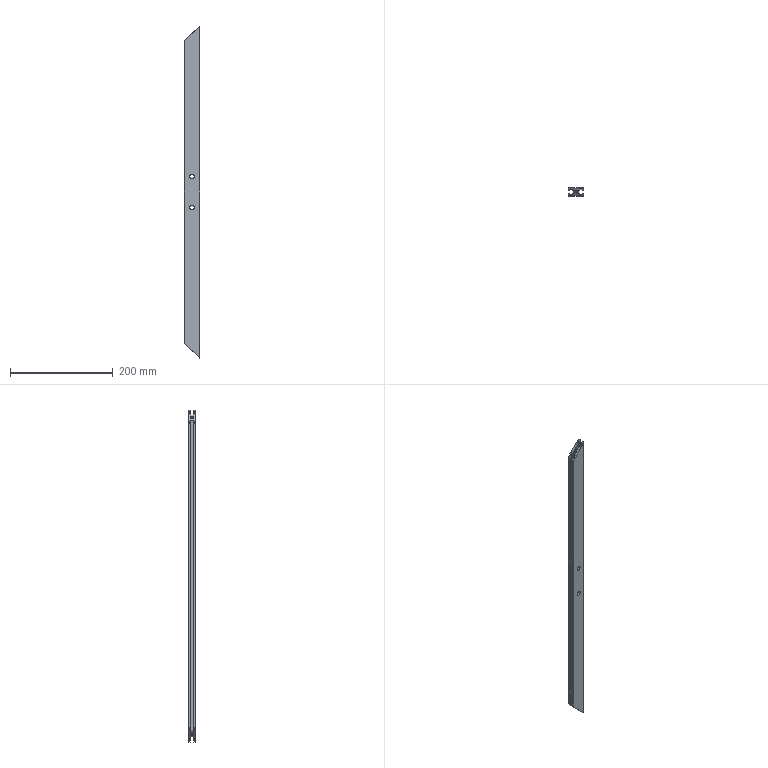Part | NX | features BREP 1 | 1 solid | 95 faces | box 30 x 15 x 647 mm | volume 147493 mm3 | plane 54 | cylinder 41 | commonest cylinder face diameters 1 x18 5 x15 2 x4 8.5 x4